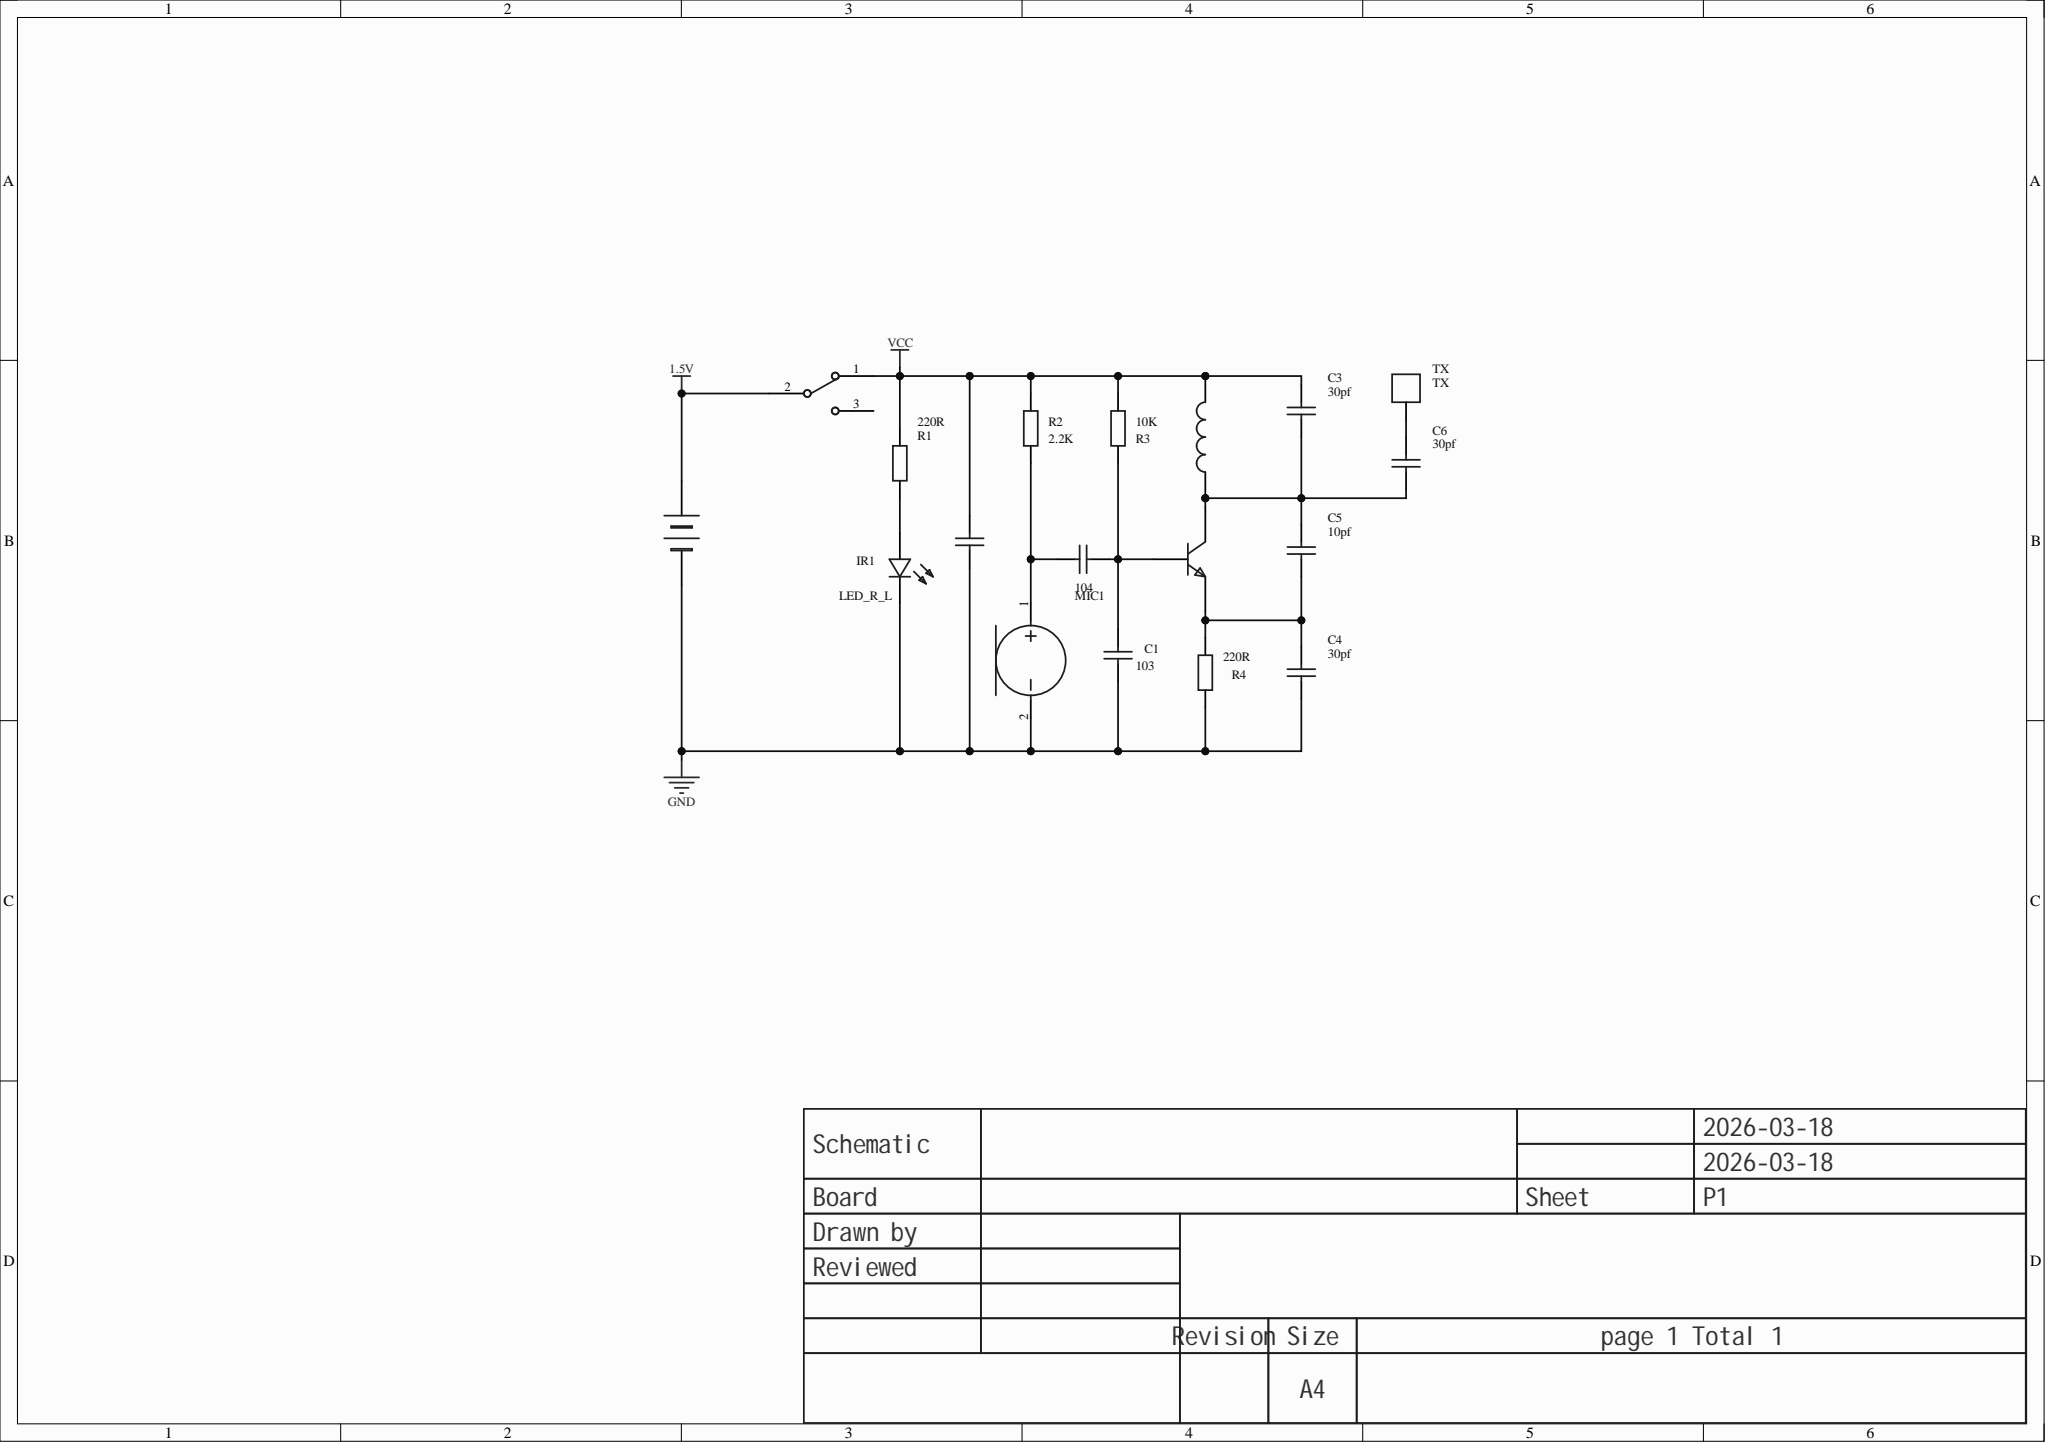Circuit board | Altium Designer | 18 parts | 9 nets
Bill of materials:
Comment,Description,Designator,Footprint,LibRef,Quantity
"BATTERY","","BT1","Bat_Box_01","BATTERY","1"
"103","","C1","CC 1.8*3.6","103","1"
"104","","C2, C7","CC 2.2*5","104","2"
"30pf","","C3, C4, C6","CC 1.8*3.6","30pf","3"
"10pf","","C5","CC 1.8*3.6","10pf","1"
"LED_R_L","","IR1","LED-TH_BD5.0-P2.54-FD","LED_R_G","1"
"4T","","L1","IND_5x5","L","1"
"MIC","","MIC1","MIC-TH_BD6.0-P1.90-D0.4-L-FD_GMI6050P-2CXXDB","MIC","1"
"9018","","Q1","TANS","9018","1"
"Res","","R1, R2, R3, R4","AXIAL0.4-1/4W","220R, 2.2K, 10K","4"
"MTS-10x","","S1","SW-TH_KH-SS12D01-G3-5.0","MTS-10x","1"
"TX","","TX","TX","TX","1"
Netlist (Protel format):
[
BT1
Bat_Box_01
BATTERY



]
[
C1
CC 1.8*3.6
103



]
[
C2
CC 2.2*5
104



]
[
C3
CC 1.8*3.6
30pf



]
[
C4
CC 1.8*3.6
30pf



]
[
C5
CC 1.8*3.6
10pf



]
[
C6
CC 1.8*3.6
30pf



]
[
C7
CC 2.2*5
104



]
[
IR1
LED-TH_BD5.0-P2.54-FD
LED_R_L



]
[
L1
IND_5x5
4T



]
[
MIC1
MIC-TH_BD6.0-P1.90-D0.4-L-FD_GMI6050P-2CXXDB
MIC



]
[
Q1
TANS
9018



]
[
R1
AXIAL0.4-1/4W
Res



]
[
R2
AXIAL0.4-1/4W
Res



]
[
R3
AXIAL0.4-1/4W
Res



]
[
R4
AXIAL0.4-1/4W
Res



]
[
S1
SW-TH_KH-SS12D01-G3-5.0
MTS-10x



]
[
TX
TX
TX



]
(
VCC
C3-2
C7-2
L1-1
R1-2
R2-2
R3-2
S1-1
)
(
NetIR1_1
IR1-1
R1-1
)
(
NetC6_2
C6-2
TX-1
)
(
NetC4_2
C4-2
C5-1
Q1-1
R4-2
)
(
NetC3_1
C3-1
C5-2
C6-1
L1-2
Q1-3
)
(
NetC2_1
C2-1
MIC1-1
R2-1
)
(
NetC1_2
C1-2
C2-2
Q1-2
R3-1
)
(
GND
BT1-2
C1-1
C4-1
C7-1
IR1-2
MIC1-2
R4-1
)
(
1.5V
BT1-1
S1-2
)